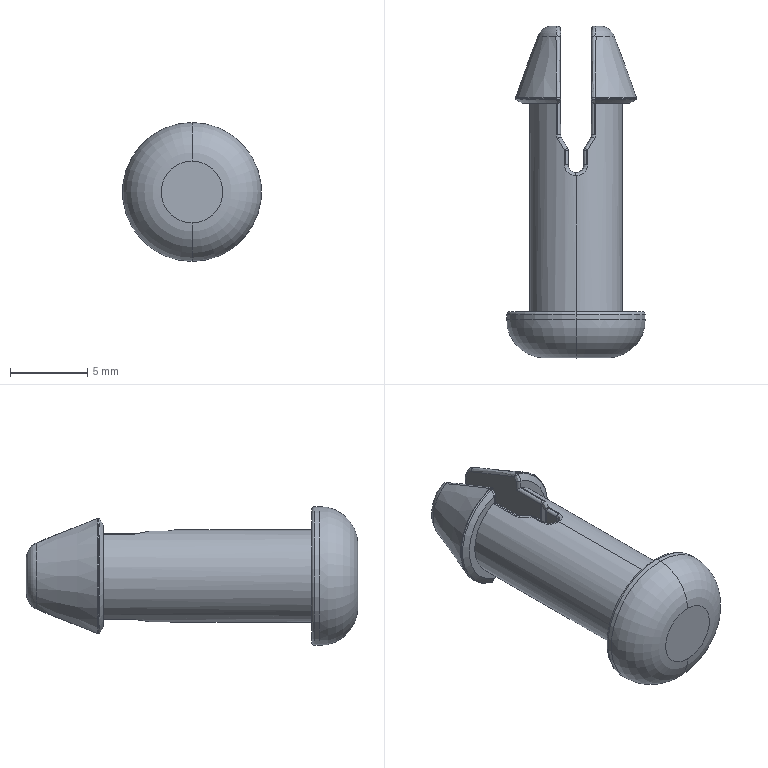Part | STEP file | 101000005926 | 1 solid | 76 faces | box 9 x 21.5 x 9 mm | volume 593.361 mm3 | spline 28 | cylinder 22 | plane 12 | torus 10 | cone 4 | commonest cylinder face diameters 0.4 x12 0.6 x4 1 x2 6 x2 9 x2